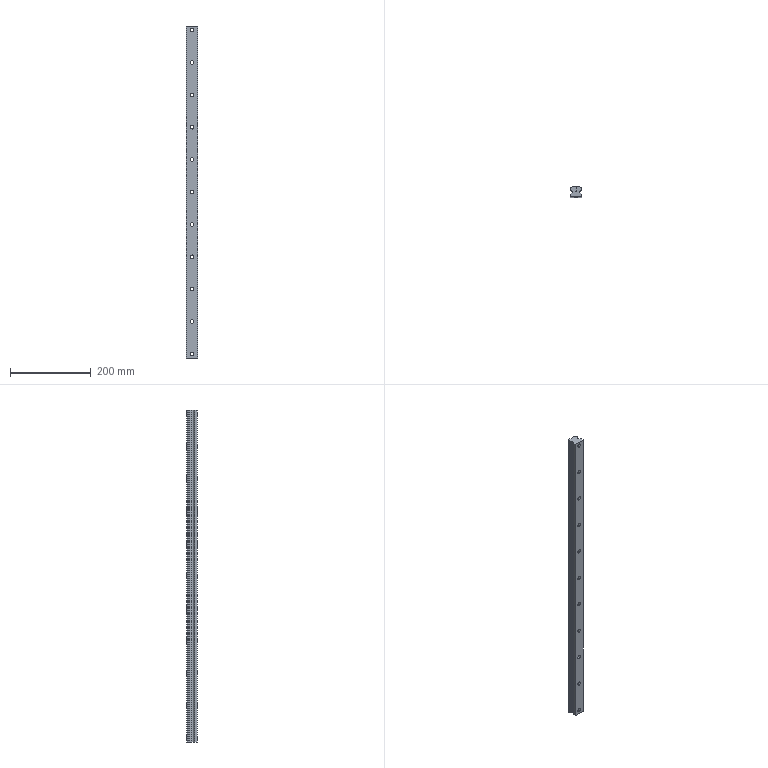Part | SolidWorks | features ICE 19, MirrorPattern 5, Extrusion 4, MirrorSolid 4, Chamfer 3, Fillet 3, RevCut 3, Dome 2, LPattern 2, DeleteBody 1, LibraryFeature 1, Revolution 1 | 1 solid | 81 faces | box 28 x 26 x 820 mm | volume 496717 mm3 | cylinder 50 | plane 31 | commonest cylinder face diameters 9 x22 14 x22 2.822 x6